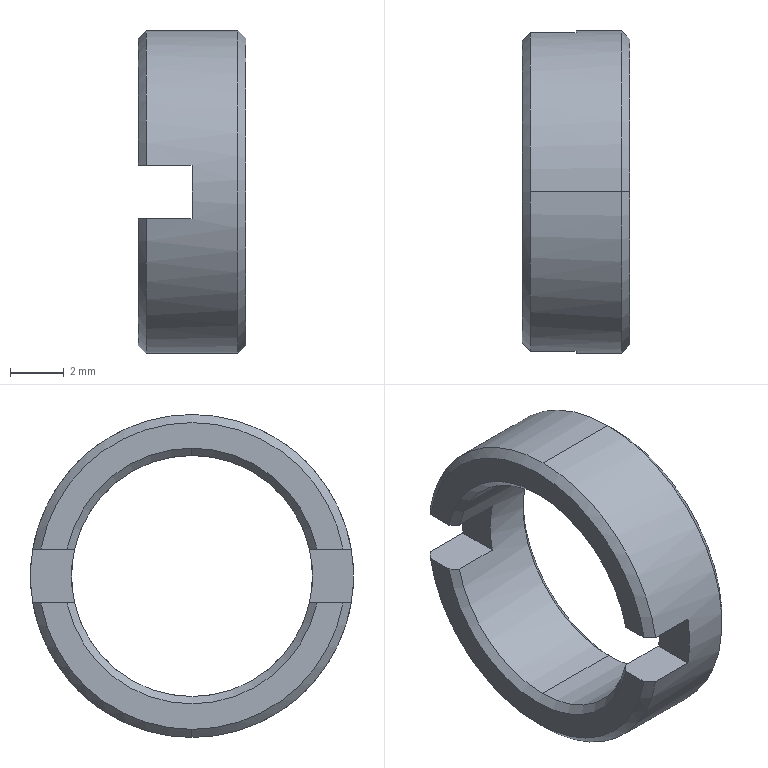Part | SolidWorks | features ICE 1, Revolution 1 | 1 solid | 23 faces | box 4 x 12 x 12 mm | volume 182.884 mm3 | cone 10 | plane 9 | cylinder 4 | commonest cylinder face diameters 8.959 x2 12 x2
STEP:
#1=CARTESIAN_POINT('',(1.7,0.,6.));
#2=VERTEX_POINT('',#1);
#3=CARTESIAN_POINT('',(1.7,0.,-6.));
#4=VERTEX_POINT('',#3);
#5=CARTESIAN_POINT('',(1.7,0.,0.));
#6=DIRECTION('',(-1.,0.,0.));
#7=DIRECTION('',(0.,0.,1.));
#8=AXIS2_PLACEMENT_3D('',#5,#6,#7);
#9=CIRCLE('',#8,6.);
#10=EDGE_CURVE('',#2,#4,#9,.T.);
#11=ORIENTED_EDGE('',*,*,#10,.T.);
#12=CARTESIAN_POINT('',(-1.7,0.,-6.));
#13=VERTEX_POINT('',#12);
#14=CARTESIAN_POINT('',(2.,0.,-6.));
#15=DIRECTION('',(-1.,0.,0.));
#16=VECTOR('',#15,1000.);
#17=LINE('',#14,#16);
#18=EDGE_CURVE('',#4,#13,#17,.T.);
#19=ORIENTED_EDGE('',*,*,#18,.T.);
#20=CARTESIAN_POINT('',(-1.7,5.916,-1.));
#21=VERTEX_POINT('',#20);
#22=CARTESIAN_POINT('',(-1.7,0.,0.));
#23=DIRECTION('',(-1.,0.,0.));
#24=DIRECTION('',(0.,0.,1.));
#25=AXIS2_PLACEMENT_3D('',#22,#23,#24);
#26=CIRCLE('',#25,6.);
#27=EDGE_CURVE('',#21,#13,#26,.T.);
#28=ORIENTED_EDGE('',*,*,#27,.F.);
#29=CARTESIAN_POINT('',(0.,5.916,-1.));
#30=VERTEX_POINT('',#29);
#31=CARTESIAN_POINT('',(2.,5.916,-1.));
#32=DIRECTION('',(-1.,0.,0.));
#33=VECTOR('',#32,1000.);
#34=LINE('',#31,#33);
#35=EDGE_CURVE('',#30,#21,#34,.T.);
#36=ORIENTED_EDGE('',*,*,#35,.F.);
#37=CARTESIAN_POINT('',(0.,5.916,1.));
#38=VERTEX_POINT('',#37);
#39=CARTESIAN_POINT('',(0.,0.,0.));
#40=DIRECTION('',(-1.,0.,0.));
#41=DIRECTION('',(0.,0.,1.));
#42=AXIS2_PLACEMENT_3D('',#39,#40,#41);
#43=CIRCLE('',#42,6.);
#44=EDGE_CURVE('',#38,#30,#43,.T.);
#45=ORIENTED_EDGE('',*,*,#44,.F.);
#46=CARTESIAN_POINT('',(-1.7,5.916,1.));
#47=VERTEX_POINT('',#46);
#48=CARTESIAN_POINT('',(2.,5.916,1.));
#49=DIRECTION('',(-1.,0.,0.));
#50=VECTOR('',#49,1000.);
#51=LINE('',#48,#50);
#52=EDGE_CURVE('',#38,#47,#51,.T.);
#53=ORIENTED_EDGE('',*,*,#52,.T.);
#54=CARTESIAN_POINT('',(-1.7,0.,6.));
#55=VERTEX_POINT('',#54);
#56=CARTESIAN_POINT('',(-1.7,0.,0.));
#57=DIRECTION('',(-1.,0.,0.));
#58=DIRECTION('',(0.,0.,1.));
#59=AXIS2_PLACEMENT_3D('',#56,#57,#58);
#60=CIRCLE('',#59,6.);
#61=EDGE_CURVE('',#55,#47,#60,.T.);
#62=ORIENTED_EDGE('',*,*,#61,.F.);
#63=CARTESIAN_POINT('',(2.,0.,6.));
#64=DIRECTION('',(-1.,0.,0.));
#65=VECTOR('',#64,1000.);
#66=LINE('',#63,#65);
#67=EDGE_CURVE('',#2,#55,#66,.T.);
#68=ORIENTED_EDGE('',*,*,#67,.F.);
#69=EDGE_LOOP('',(#11,#19,#28,#36,#45,#53,#62,#68));
#70=FACE_OUTER_BOUND('',#69,.T.);
#71=CARTESIAN_POINT('',(2.,0.,0.));
#72=DIRECTION('',(-1.,0.,0.));
#73=DIRECTION('',(0.,0.,1.));
#74=AXIS2_PLACEMENT_3D('',#71,#72,#73);
#75=CYLINDRICAL_SURFACE('',#74,6.);
#76=ADVANCED_FACE('',(#70),#75,.T.);
#77=CARTESIAN_POINT('',(2.,0.,5.7));
#78=VERTEX_POINT('',#77);
#79=CARTESIAN_POINT('',(2.,0.,-5.7));
#80=VERTEX_POINT('',#79);
#81=CARTESIAN_POINT('',(2.,0.,0.));
#82=DIRECTION('',(-1.,0.,0.));
#83=DIRECTION('',(0.,0.,1.));
#84=AXIS2_PLACEMENT_3D('',#81,#82,#83);
#85=CIRCLE('',#84,5.7);
#86=EDGE_CURVE('',#78,#80,#85,.T.);
#87=ORIENTED_EDGE('',*,*,#86,.T.);
#88=CARTESIAN_POINT('',(2.,0.,-5.7));
#89=DIRECTION('',(-0.7071,0.,-0.7071));
#90=VECTOR('',#89,1000.);
#91=LINE('',#88,#90);
#92=EDGE_CURVE('',#80,#4,#91,.T.);
#93=ORIENTED_EDGE('',*,*,#92,.T.);
#94=ORIENTED_EDGE('',*,*,#10,.F.);
#95=CARTESIAN_POINT('',(2.,0.,5.7));
#96=DIRECTION('',(-0.7071,0.,0.7071));
#97=VECTOR('',#96,1000.);
#98=LINE('',#95,#97);
#99=EDGE_CURVE('',#78,#2,#98,.T.);
#100=ORIENTED_EDGE('',*,*,#99,.F.);
#101=EDGE_LOOP('',(#87,#93,#94,#100));
#102=FACE_OUTER_BOUND('',#101,.T.);
#103=CARTESIAN_POINT('',(2.,0.,0.));
#104=DIRECTION('',(-1.,0.,0.));
#105=DIRECTION('',(0.,0.,1.));
#106=AXIS2_PLACEMENT_3D('',#103,#104,#105);
#107=CONICAL_SURFACE('',#106,5.7,0.7854);
#108=ADVANCED_FACE('',(#102),#107,.T.);
#109=CARTESIAN_POINT('',(1.729,0.,-4.479));
#110=VERTEX_POINT('',#109);
#111=CARTESIAN_POINT('',(1.729,0.,4.479));
#112=VERTEX_POINT('',#111);
#113=CARTESIAN_POINT('',(1.729,0.,0.));
#114=DIRECTION('',(-1.,0.,0.));
#115=DIRECTION('',(0.,0.,1.));
#116=AXIS2_PLACEMENT_3D('',#113,#114,#115);
#117=CIRCLE('',#116,4.479);
#118=EDGE_CURVE('',#110,#112,#117,.T.);
#119=ORIENTED_EDGE('',*,*,#118,.T.);
#120=CARTESIAN_POINT('',(2.,0.,4.75));
#121=VERTEX_POINT('',#120);
#122=CARTESIAN_POINT('',(1.729,0.,4.479));
#123=DIRECTION('',(0.7071,0.,0.7071));
#124=VECTOR('',#123,1000.);
#125=LINE('',#122,#124);
#126=EDGE_CURVE('',#112,#121,#125,.T.);
#127=ORIENTED_EDGE('',*,*,#126,.T.);
#128=CARTESIAN_POINT('',(2.,0.,-4.75));
#129=VERTEX_POINT('',#128);
#130=CARTESIAN_POINT('',(2.,0.,0.));
#131=DIRECTION('',(-1.,0.,0.));
#132=DIRECTION('',(0.,0.,1.));
#133=AXIS2_PLACEMENT_3D('',#130,#131,#132);
#134=CIRCLE('',#133,4.75);
#135=EDGE_CURVE('',#129,#121,#134,.T.);
#136=ORIENTED_EDGE('',*,*,#135,.F.);
#137=CARTESIAN_POINT('',(1.729,0.,-4.479));
#138=DIRECTION('',(0.7071,0.,-0.7071));
#139=VECTOR('',#138,1000.);
#140=LINE('',#137,#139);
#141=EDGE_CURVE('',#110,#129,#140,.T.);
#142=ORIENTED_EDGE('',*,*,#141,.F.);
#143=EDGE_LOOP('',(#119,#127,#136,#142));
#144=FACE_OUTER_BOUND('',#143,.T.);
#145=CARTESIAN_POINT('',(1.729,0.,0.));
#146=DIRECTION('',(1.,0.,0.));
#147=DIRECTION('',(0.,0.,-1.));
#148=AXIS2_PLACEMENT_3D('',#145,#146,#147);
#149=CONICAL_SURFACE('',#148,4.479,0.7854);
#150=ADVANCED_FACE('',(#144),#149,.F.);
#151=ORIENTED_EDGE('',*,*,#118,.F.);
#152=CARTESIAN_POINT('',(-1.73,0.,-4.479));
#153=VERTEX_POINT('',#152);
#154=CARTESIAN_POINT('',(2.,0.,-4.479));
#155=DIRECTION('',(-1.,0.,0.));
#156=VECTOR('',#155,1000.);
#157=LINE('',#154,#156);
#158=EDGE_CURVE('',#110,#153,#157,.T.);
#159=ORIENTED_EDGE('',*,*,#158,.T.);
#160=CARTESIAN_POINT('',(-1.73,-4.366,-1.));
#161=VERTEX_POINT('',#160);
#162=CARTESIAN_POINT('',(-1.73,0.,0.));
#163=DIRECTION('',(-1.,0.,0.));
#164=DIRECTION('',(0.,0.,1.));
#165=AXIS2_PLACEMENT_3D('',#162,#163,#164);
#166=CIRCLE('',#165,4.479);
#167=EDGE_CURVE('',#153,#161,#166,.T.);
#168=ORIENTED_EDGE('',*,*,#167,.T.);
#169=CARTESIAN_POINT('',(0.,-4.366,-1.));
#170=VERTEX_POINT('',#169);
#171=CARTESIAN_POINT('',(2.,-4.366,-1.));
#172=DIRECTION('',(-1.,0.,0.));
#173=VECTOR('',#172,1000.);
#174=LINE('',#171,#173);
#175=EDGE_CURVE('',#170,#161,#174,.T.);
#176=ORIENTED_EDGE('',*,*,#175,.F.);
#177=CARTESIAN_POINT('',(0.,-4.366,1.));
#178=VERTEX_POINT('',#177);
#179=CARTESIAN_POINT('',(0.,0.,0.));
#180=DIRECTION('',(1.,0.,0.));
#181=DIRECTION('',(0.,0.,1.));
#182=AXIS2_PLACEMENT_3D('',#179,#180,#181);
#183=CIRCLE('',#182,4.479);
#184=EDGE_CURVE('',#178,#170,#183,.T.);
#185=ORIENTED_EDGE('',*,*,#184,.F.);
#186=CARTESIAN_POINT('',(-1.73,-4.366,1.));
#187=VERTEX_POINT('',#186);
#188=CARTESIAN_POINT('',(2.,-4.366,1.));
#189=DIRECTION('',(-1.,0.,0.));
#190=VECTOR('',#189,1000.);
#191=LINE('',#188,#190);
#192=EDGE_CURVE('',#178,#187,#191,.T.);
#193=ORIENTED_EDGE('',*,*,#192,.T.);
#194=CARTESIAN_POINT('',(-1.73,0.,4.479));
#195=VERTEX_POINT('',#194);
#196=CARTESIAN_POINT('',(-1.73,0.,0.));
#197=DIRECTION('',(-1.,0.,0.));
#198=DIRECTION('',(0.,0.,1.));
#199=AXIS2_PLACEMENT_3D('',#196,#197,#198);
#200=CIRCLE('',#199,4.479);
#201=EDGE_CURVE('',#187,#195,#200,.T.);
#202=ORIENTED_EDGE('',*,*,#201,.T.);
#203=CARTESIAN_POINT('',(2.,0.,4.479));
#204=DIRECTION('',(-1.,0.,0.));
#205=VECTOR('',#204,1000.);
#206=LINE('',#203,#205);
#207=EDGE_CURVE('',#112,#195,#206,.T.);
#208=ORIENTED_EDGE('',*,*,#207,.F.);
#209=EDGE_LOOP('',(#151,#159,#168,#176,#185,#193,#202,#208));
#210=FACE_OUTER_BOUND('',#209,.T.);
#211=CARTESIAN_POINT('',(2.,0.,0.));
#212=DIRECTION('',(-1.,0.,0.));
#213=DIRECTION('',(0.,0.,1.));
#214=AXIS2_PLACEMENT_3D('',#211,#212,#213);
#215=CYLINDRICAL_SURFACE('',#214,4.479);
#216=ADVANCED_FACE('',(#210),#215,.F.);
#217=CARTESIAN_POINT('',(-1.73,4.366,1.));
#218=VERTEX_POINT('',#217);
#219=CARTESIAN_POINT('',(-1.73,0.,0.));
#220=DIRECTION('',(-1.,0.,0.));
#221=DIRECTION('',(0.,0.,1.));
#222=AXIS2_PLACEMENT_3D('',#219,#220,#221);
#223=CIRCLE('',#222,4.479);
#224=EDGE_CURVE('',#195,#218,#223,.T.);
#225=ORIENTED_EDGE('',*,*,#224,.F.);
#226=CARTESIAN_POINT('',(-2.,0.,4.75));
#227=VERTEX_POINT('',#226);
#228=CARTESIAN_POINT('',(-2.,0.,4.75));
#229=DIRECTION('',(-0.7071,0.,0.7071));
#230=VECTOR('',#229,1000.);
#231=LINE('',#228,#230);
#232=EDGE_CURVE('',#195,#227,#231,.T.);
#233=ORIENTED_EDGE('',*,*,#232,.T.);
#234=CARTESIAN_POINT('',(-2.,4.644,1.));
#235=VERTEX_POINT('',#234);
#236=CARTESIAN_POINT('',(-2.,0.,0.));
#237=DIRECTION('',(-1.,0.,0.));
#238=DIRECTION('',(0.,0.,1.));
#239=AXIS2_PLACEMENT_3D('',#236,#237,#238);
#240=CIRCLE('',#239,4.75);
#241=EDGE_CURVE('',#227,#235,#240,.T.);
#242=ORIENTED_EDGE('',*,*,#241,.T.);
#243=CARTESIAN_POINT('',(-2.,4.644,1.));
#244=CARTESIAN_POINT('',(-1.91,4.551,1.));
#245=CARTESIAN_POINT('',(-1.82,4.459,1.));
#246=CARTESIAN_POINT('',(-1.73,4.366,1.));
#247=B_SPLINE_CURVE_WITH_KNOTS('',3,(#243,#244,#245,#246),.UNSPECIFIED.,.F.,.F.,(4,4),(0.000001,0.0003876),.UNSPECIFIED.);
#248=EDGE_CURVE('',#235,#218,#247,.T.);
#249=ORIENTED_EDGE('',*,*,#248,.T.);
#250=EDGE_LOOP('',(#225,#233,#242,#249));
#251=FACE_OUTER_BOUND('',#250,.T.);
#252=CARTESIAN_POINT('',(-2.,0.,0.));
#253=DIRECTION('',(-1.,0.,0.));
#254=DIRECTION('',(0.,0.,1.));
#255=AXIS2_PLACEMENT_3D('',#252,#253,#254);
#256=CONICAL_SURFACE('',#255,4.75,0.7854);
#257=ADVANCED_FACE('',(#251),#256,.F.);
#258=CARTESIAN_POINT('',(-2.,0.,-5.7));
#259=VERTEX_POINT('',#258);
#260=CARTESIAN_POINT('',(-2.,-5.612,-1.));
#261=VERTEX_POINT('',#260);
#262=CARTESIAN_POINT('',(-2.,0.,0.));
#263=DIRECTION('',(-1.,0.,0.));
#264=DIRECTION('',(0.,0.,1.));
#265=AXIS2_PLACEMENT_3D('',#262,#263,#264);
#266=CIRCLE('',#265,5.7);
#267=EDGE_CURVE('',#259,#261,#266,.T.);
#268=ORIENTED_EDGE('',*,*,#267,.F.);
#269=CARTESIAN_POINT('',(-1.7,0.,-6.));
#270=DIRECTION('',(0.7071,0.,-0.7071));
#271=VECTOR('',#270,1000.);
#272=LINE('',#269,#271);
#273=EDGE_CURVE('',#259,#13,#272,.T.);
#274=ORIENTED_EDGE('',*,*,#273,.T.);
#275=CARTESIAN_POINT('',(-1.7,-5.916,-1.));
#276=VERTEX_POINT('',#275);
#277=CARTESIAN_POINT('',(-1.7,0.,0.));
#278=DIRECTION('',(-1.,0.,0.));
#279=DIRECTION('',(0.,0.,1.));
#280=AXIS2_PLACEMENT_3D('',#277,#278,#279);
#281=CIRCLE('',#280,6.);
#282=EDGE_CURVE('',#13,#276,#281,.T.);
#283=ORIENTED_EDGE('',*,*,#282,.T.);
#284=CARTESIAN_POINT('',(-2.,-5.612,-1.));
#285=CARTESIAN_POINT('',(-1.9,-5.713,-1.));
#286=CARTESIAN_POINT('',(-1.8,-5.815,-1.));
#287=CARTESIAN_POINT('',(-1.7,-5.916,-1.));
#288=B_SPLINE_CURVE_WITH_KNOTS('',3,(#284,#285,#286,#287),.UNSPECIFIED.,.F.,.F.,(4,4),(0.01512,0.01555),.UNSPECIFIED.);
#289=EDGE_CURVE('',#261,#276,#288,.T.);
#290=ORIENTED_EDGE('',*,*,#289,.F.);
#291=EDGE_LOOP('',(#268,#274,#283,#290));
#292=FACE_OUTER_BOUND('',#291,.T.);
#293=CARTESIAN_POINT('',(-1.7,0.,0.));
#294=DIRECTION('',(1.,0.,0.));
#295=DIRECTION('',(0.,0.,-1.));
#296=AXIS2_PLACEMENT_3D('',#293,#294,#295);
#297=CONICAL_SURFACE('',#296,6.,0.7854);
#298=ADVANCED_FACE('',(#292),#297,.T.);
#299=CARTESIAN_POINT('',(-2.,5.612,-1.));
#300=VERTEX_POINT('',#299);
#301=CARTESIAN_POINT('',(-2.,4.644,-1.));
#302=VERTEX_POINT('',#301);
#303=CARTESIAN_POINT('',(-2.,5.7,-1.));
#304=DIRECTION('',(0.,-1.,0.));
#305=VECTOR('',#304,1000.);
#306=LINE('',#303,#305);
#307=EDGE_CURVE('',#300,#302,#306,.T.);
#308=ORIENTED_EDGE('',*,*,#307,.F.);
#309=CARTESIAN_POINT('',(-2.,0.,0.));
#310=DIRECTION('',(-1.,0.,0.));
#311=DIRECTION('',(0.,0.,1.));
#312=AXIS2_PLACEMENT_3D('',#309,#310,#311);
#313=CIRCLE('',#312,5.7);
#314=EDGE_CURVE('',#300,#259,#313,.T.);
#315=ORIENTED_EDGE('',*,*,#314,.T.);
#316=ORIENTED_EDGE('',*,*,#267,.T.);
#317=CARTESIAN_POINT('',(-2.,-4.644,-1.));
#318=VERTEX_POINT('',#317);
#319=CARTESIAN_POINT('',(-2.,5.7,-1.));
#320=DIRECTION('',(0.,-1.,0.));
#321=VECTOR('',#320,1000.);
#322=LINE('',#319,#321);
#323=EDGE_CURVE('',#318,#261,#322,.T.);
#324=ORIENTED_EDGE('',*,*,#323,.F.);
#325=CARTESIAN_POINT('',(-2.,0.,0.));
#326=DIRECTION('',(-1.,0.,0.));
#327=DIRECTION('',(0.,0.,1.));
#328=AXIS2_PLACEMENT_3D('',#325,#326,#327);
#329=CIRCLE('',#328,4.75);
#330=EDGE_CURVE('',#302,#318,#329,.T.);
#331=ORIENTED_EDGE('',*,*,#330,.F.);
#332=EDGE_LOOP('',(#308,#315,#316,#324,#331));
#333=FACE_OUTER_BOUND('',#332,.T.);
#334=CARTESIAN_POINT('',(-2.,5.7,0.));
#335=DIRECTION('',(1.,0.,0.));
#336=DIRECTION('',(0.,0.,-1.));
#337=AXIS2_PLACEMENT_3D('',#334,#335,#336);
#338=PLANE('',#337);
#339=ADVANCED_FACE('',(#333),#338,.F.);
#340=CARTESIAN_POINT('',(-1.73,4.366,-1.));
#341=VERTEX_POINT('',#340);
#342=CARTESIAN_POINT('',(-2.,4.644,-1.));
#343=CARTESIAN_POINT('',(-1.91,4.551,-1.));
#344=CARTESIAN_POINT('',(-1.82,4.459,-1.));
#345=CARTESIAN_POINT('',(-1.73,4.366,-1.));
#346=B_SPLINE_CURVE_WITH_KNOTS('',3,(#342,#343,#344,#345),.UNSPECIFIED.,.F.,.F.,(4,4),(0.000001,0.0003876),.UNSPECIFIED.);
#347=EDGE_CURVE('',#302,#341,#346,.T.);
#348=ORIENTED_EDGE('',*,*,#347,.F.);
#349=ORIENTED_EDGE('',*,*,#330,.T.);
#350=CARTESIAN_POINT('',(-1.73,-4.366,-1.));
#351=CARTESIAN_POINT('',(-1.82,-4.459,-1.));
#352=CARTESIAN_POINT('',(-1.91,-4.551,-1.));
#353=CARTESIAN_POINT('',(-2.,-4.644,-1.));
#354=B_SPLINE_CURVE_WITH_KNOTS('',3,(#350,#351,#352,#353),.UNSPECIFIED.,.F.,.F.,(4,4),(0.01142,0.01179),.UNSPECIFIED.);
#355=EDGE_CURVE('',#161,#318,#354,.T.);
#356=ORIENTED_EDGE('',*,*,#355,.F.);
#357=ORIENTED_EDGE('',*,*,#167,.F.);
#358=CARTESIAN_POINT('',(-1.73,0.,0.));
#359=DIRECTION('',(-1.,0.,0.));
#360=DIRECTION('',(0.,0.,1.));
#361=AXIS2_PLACEMENT_3D('',#358,#359,#360);
#362=CIRCLE('',#361,4.479);
#363=EDGE_CURVE('',#341,#153,#362,.T.);
#364=ORIENTED_EDGE('',*,*,#363,.F.);
#365=EDGE_LOOP('',(#348,#349,#356,#357,#364));
#366=FACE_OUTER_BOUND('',#365,.T.);
#367=CARTESIAN_POINT('',(-2.,0.,0.));
#368=DIRECTION('',(-1.,0.,0.));
#369=DIRECTION('',(0.,0.,1.));
#370=AXIS2_PLACEMENT_3D('',#367,#368,#369);
#371=CONICAL_SURFACE('',#370,4.75,0.7854);
#372=ADVANCED_FACE('',(#366),#371,.F.);
#373=ORIENTED_EDGE('',*,*,#273,.F.);
#374=ORIENTED_EDGE('',*,*,#314,.F.);
#375=CARTESIAN_POINT('',(-1.7,5.916,-1.));
#376=CARTESIAN_POINT('',(-1.8,5.815,-1.));
#377=CARTESIAN_POINT('',(-1.9,5.713,-1.));
#378=CARTESIAN_POINT('',(-2.,5.612,-1.));
#379=B_SPLINE_CURVE_WITH_KNOTS('',3,(#375,#376,#377,#378),.UNSPECIFIED.,.F.,.F.,(4,4),(0.000000996,0.0004282),.UNSPECIFIED.);
#380=EDGE_CURVE('',#21,#300,#379,.T.);
#381=ORIENTED_EDGE('',*,*,#380,.F.);
#382=ORIENTED_EDGE('',*,*,#27,.T.);
#383=EDGE_LOOP('',(#373,#374,#381,#382));
#384=FACE_OUTER_BOUND('',#383,.T.);
#385=CARTESIAN_POINT('',(-1.7,0.,0.));
#386=DIRECTION('',(1.,0.,0.));
#387=DIRECTION('',(0.,0.,-1.));
#388=AXIS2_PLACEMENT_3D('',#385,#386,#387);
#389=CONICAL_SURFACE('',#388,6.,0.7854);
#390=ADVANCED_FACE('',(#384),#389,.T.);
#391=CARTESIAN_POINT('',(-2.,-5.612,1.));
#392=VERTEX_POINT('',#391);
#393=CARTESIAN_POINT('',(-2.,5.612,1.));
#394=VERTEX_POINT('',#393);
#395=CARTESIAN_POINT('',(-2.,0.,0.));
#396=DIRECTION('',(-1.,0.,0.));
#397=DIRECTION('',(0.,0.,1.));
#398=AXIS2_PLACEMENT_3D('',#395,#396,#397);
#399=CIRCLE('',#398,5.7);
#400=EDGE_CURVE('',#392,#394,#399,.T.);
#401=ORIENTED_EDGE('',*,*,#400,.T.);
#402=CARTESIAN_POINT('',(-2.,5.7,1.));
#403=DIRECTION('',(0.,-1.,0.));
#404=VECTOR('',#403,1000.);
#405=LINE('',#402,#404);
#406=EDGE_CURVE('',#394,#235,#405,.T.);
#407=ORIENTED_EDGE('',*,*,#406,.T.);
#408=ORIENTED_EDGE('',*,*,#241,.F.);
#409=CARTESIAN_POINT('',(-2.,-4.644,1.));
#410=VERTEX_POINT('',#409);
#411=CARTESIAN_POINT('',(-2.,0.,0.));
#412=DIRECTION('',(-1.,0.,0.));
#413=DIRECTION('',(0.,0.,1.));
#414=AXIS2_PLACEMENT_3D('',#411,#412,#413);
#415=CIRCLE('',#414,4.75);
#416=EDGE_CURVE('',#410,#227,#415,.T.);
#417=ORIENTED_EDGE('',*,*,#416,.F.);
#418=CARTESIAN_POINT('',(-2.,5.7,1.));
#419=DIRECTION('',(0.,-1.,0.));
#420=VECTOR('',#419,1000.);
#421=LINE('',#418,#420);
#422=EDGE_CURVE('',#410,#392,#421,.T.);
#423=ORIENTED_EDGE('',*,*,#422,.T.);
#424=EDGE_LOOP('',(#401,#407,#408,#417,#423));
#425=FACE_OUTER_BOUND('',#424,.T.);
#426=CARTESIAN_POINT('',(-2.,5.7,0.));
#427=DIRECTION('',(1.,0.,0.));
#428=DIRECTION('',(0.,0.,-1.));
#429=AXIS2_PLACEMENT_3D('',#426,#427,#428);
#430=PLANE('',#429);
#431=ADVANCED_FACE('',(#425),#430,.F.);
#432=ORIENTED_EDGE('',*,*,#232,.F.);
#433=ORIENTED_EDGE('',*,*,#201,.F.);
#434=CARTESIAN_POINT('',(-1.73,-4.366,1.));
#435=CARTESIAN_POINT('',(-1.82,-4.459,1.));
#436=CARTESIAN_POINT('',(-1.91,-4.551,1.));
#437=CARTESIAN_POINT('',(-2.,-4.644,1.));
#438=B_SPLINE_CURVE_WITH_KNOTS('',3,(#434,#435,#436,#437),.UNSPECIFIED.,.F.,.F.,(4,4),(0.01142,0.01179),.UNSPECIFIED.);
#439=EDGE_CURVE('',#187,#410,#438,.T.);
#440=ORIENTED_EDGE('',*,*,#439,.T.);
#441=ORIENTED_EDGE('',*,*,#416,.T.);
#442=EDGE_LOOP('',(#432,#433,#440,#441));
#443=FACE_OUTER_BOUND('',#442,.T.);
#444=CARTESIAN_POINT('',(-2.,0.,0.));
#445=DIRECTION('',(-1.,0.,0.));
#446=DIRECTION('',(0.,0.,1.));
#447=AXIS2_PLACEMENT_3D('',#444,#445,#446);
#448=CONICAL_SURFACE('',#447,4.75,0.7854);
#449=ADVANCED_FACE('',(#443),#448,.F.);
#450=ORIENTED_EDGE('',*,*,#158,.F.);
#451=CARTESIAN_POINT('',(1.729,0.,0.));
#452=DIRECTION('',(-1.,0.,0.));
#453=DIRECTION('',(0.,0.,1.));
#454=AXIS2_PLACEMENT_3D('',#451,#452,#453);
#455=CIRCLE('',#454,4.479);
#456=EDGE_CURVE('',#112,#110,#455,.T.);
#457=ORIENTED_EDGE('',*,*,#456,.F.);
#458=ORIENTED_EDGE('',*,*,#207,.T.);
#459=ORIENTED_EDGE('',*,*,#224,.T.);
#460=CARTESIAN_POINT('',(0.,4.366,1.));
#461=VERTEX_POINT('',#460);
#462=CARTESIAN_POINT('',(2.,4.366,1.));
#463=DIRECTION('',(1.,0.,0.));
#464=VECTOR('',#463,1000.);
#465=LINE('',#462,#464);
#466=EDGE_CURVE('',#218,#461,#465,.T.);
#467=ORIENTED_EDGE('',*,*,#466,.T.);
#468=CARTESIAN_POINT('',(0.,4.366,-1.));
#469=VERTEX_POINT('',#468);
#470=CARTESIAN_POINT('',(0.,0.,0.));
#471=DIRECTION('',(1.,0.,0.));
#472=DIRECTION('',(0.,0.,1.));
#473=AXIS2_PLACEMENT_3D('',#470,#471,#472);
#474=CIRCLE('',#473,4.479);
#475=EDGE_CURVE('',#469,#461,#474,.T.);
#476=ORIENTED_EDGE('',*,*,#475,.F.);
#477=CARTESIAN_POINT('',(2.,4.366,-1.));
#478=DIRECTION('',(1.,0.,0.));
#479=VECTOR('',#478,1000.);
#480=LINE('',#477,#479);
#481=EDGE_CURVE('',#341,#469,#480,.T.);
#482=ORIENTED_EDGE('',*,*,#481,.F.);
#483=ORIENTED_EDGE('',*,*,#363,.T.);
#484=EDGE_LOOP('',(#450,#457,#458,#459,#467,#476,#482,#483));
#485=FACE_OUTER_BOUND('',#484,.T.);
#486=CARTESIAN_POINT('',(2.,0.,0.));
#487=DIRECTION('',(-1.,0.,0.));
#488=DIRECTION('',(0.,0.,1.));
#489=AXIS2_PLACEMENT_3D('',#486,#487,#488);
#490=CYLINDRICAL_SURFACE('',#489,4.479);
#491=ADVANCED_FACE('',(#485),#490,.F.);
#492=ORIENTED_EDGE('',*,*,#126,.F.);
#493=ORIENTED_EDGE('',*,*,#456,.T.);
#494=ORIENTED_EDGE('',*,*,#141,.T.);
#495=CARTESIAN_POINT('',(2.,0.,0.));
#496=DIRECTION('',(-1.,0.,0.));
#497=DIRECTION('',(0.,0.,1.));
#498=AXIS2_PLACEMENT_3D('',#495,#496,#497);
#499=CIRCLE('',#498,4.75);
#500=EDGE_CURVE('',#121,#129,#499,.T.);
#501=ORIENTED_EDGE('',*,*,#500,.F.);
#502=EDGE_LOOP('',(#492,#493,#494,#501));
#503=FACE_OUTER_BOUND('',#502,.T.);
#504=CARTESIAN_POINT('',(1.729,0.,0.));
#505=DIRECTION('',(1.,0.,0.));
#506=DIRECTION('',(0.,0.,-1.));
#507=AXIS2_PLACEMENT_3D('',#504,#505,#506);
#508=CONICAL_SURFACE('',#507,4.479,0.7854);
#509=ADVANCED_FACE('',(#503),#508,.F.);
#510=ORIENTED_EDGE('',*,*,#86,.F.);
#511=CARTESIAN_POINT('',(2.,0.,0.));
#512=DIRECTION('',(-1.,0.,0.));
#513=DIRECTION('',(0.,0.,1.));
#514=AXIS2_PLACEMENT_3D('',#511,#512,#513);
#515=CIRCLE('',#514,5.7);
#516=EDGE_CURVE('',#80,#78,#515,.T.);
#517=ORIENTED_EDGE('',*,*,#516,.F.);
#518=EDGE_LOOP('',(#510,#517));
#519=FACE_OUTER_BOUND('',#518,.T.);
#520=ORIENTED_EDGE('',*,*,#135,.T.);
#521=ORIENTED_EDGE('',*,*,#500,.T.);
#522=EDGE_LOOP('',(#520,#521));
#523=FACE_BOUND('',#522,.T.);
#524=CARTESIAN_POINT('',(2.,4.75,0.));
#525=DIRECTION('',(-1.,0.,0.));
#526=DIRECTION('',(0.,0.,1.));
#527=AXIS2_PLACEMENT_3D('',#524,#525,#526);
#528=PLANE('',#527);
#529=ADVANCED_FACE('',(#519,#523),#528,.F.);
#530=ORIENTED_EDGE('',*,*,#92,.F.);
#531=ORIENTED_EDGE('',*,*,#516,.T.);
#532=ORIENTED_EDGE('',*,*,#99,.T.);
#533=CARTESIAN_POINT('',(1.7,0.,0.));
#534=DIRECTION('',(-1.,0.,0.));
#535=DIRECTION('',(0.,0.,1.));
#536=AXIS2_PLACEMENT_3D('',#533,#534,#535);
#537=CIRCLE('',#536,6.);
#538=EDGE_CURVE('',#4,#2,#537,.T.);
#539=ORIENTED_EDGE('',*,*,#538,.F.);
#540=EDGE_LOOP('',(#530,#531,#532,#539));
#541=FACE_OUTER_BOUND('',#540,.T.);
#542=CARTESIAN_POINT('',(2.,0.,0.));
#543=DIRECTION('',(-1.,0.,0.));
#544=DIRECTION('',(0.,0.,1.));
#545=AXIS2_PLACEMENT_3D('',#542,#543,#544);
#546=CONICAL_SURFACE('',#545,5.7,0.7854);
#547=ADVANCED_FACE('',(#541),#546,.T.);
#548=ORIENTED_EDGE('',*,*,#18,.F.);
#549=ORIENTED_EDGE('',*,*,#538,.T.);
#550=ORIENTED_EDGE('',*,*,#67,.T.);
#551=CARTESIAN_POINT('',(-1.7,-5.916,1.));
#552=VERTEX_POINT('',#551);
#553=CARTESIAN_POINT('',(-1.7,0.,0.));
#554=DIRECTION('',(-1.,0.,0.));
#555=DIRECTION('',(0.,0.,1.));
#556=AXIS2_PLACEMENT_3D('',#553,#554,#555);
#557=CIRCLE('',#556,6.);
#558=EDGE_CURVE('',#552,#55,#557,.T.);
#559=ORIENTED_EDGE('',*,*,#558,.F.);
#560=CARTESIAN_POINT('',(0.,-5.916,1.));
#561=VERTEX_POINT('',#560);
#562=CARTESIAN_POINT('',(2.,-5.916,1.));
#563=DIRECTION('',(1.,0.,0.));
#564=VECTOR('',#563,1000.);
#565=LINE('',#562,#564);
#566=EDGE_CURVE('',#552,#561,#565,.T.);
#567=ORIENTED_EDGE('',*,*,#566,.T.);
#568=CARTESIAN_POINT('',(0.,-5.916,-1.));
#569=VERTEX_POINT('',#568);
#570=CARTESIAN_POINT('',(0.,0.,0.));
#571=DIRECTION('',(-1.,0.,0.));
#572=DIRECTION('',(0.,0.,1.));
#573=AXIS2_PLACEMENT_3D('',#570,#571,#572);
#574=CIRCLE('',#573,6.);
#575=EDGE_CURVE('',#569,#561,#574,.T.);
#576=ORIENTED_EDGE('',*,*,#575,.F.);
#577=CARTESIAN_POINT('',(2.,-5.916,-1.));
#578=DIRECTION('',(1.,0.,0.));
#579=VECTOR('',#578,1000.);
#580=LINE('',#577,#579);
#581=EDGE_CURVE('',#276,#569,#580,.T.);
#582=ORIENTED_EDGE('',*,*,#581,.F.);
#583=ORIENTED_EDGE('',*,*,#282,.F.);
#584=EDGE_LOOP('',(#548,#549,#550,#559,#567,#576,#582,#583));
#585=FACE_OUTER_BOUND('',#584,.T.);
#586=CARTESIAN_POINT('',(2.,0.,0.));
#587=DIRECTION('',(-1.,0.,0.));
#588=DIRECTION('',(0.,0.,1.));
#589=AXIS2_PLACEMENT_3D('',#586,#587,#588);
#590=CYLINDRICAL_SURFACE('',#589,6.);
#591=ADVANCED_FACE('',(#585),#590,.T.);
#592=ORIENTED_EDGE('',*,*,#558,.T.);
#593=ORIENTED_EDGE('',*,*,#61,.T.);
#594=CARTESIAN_POINT('',(-1.7,5.916,1.));
#595=CARTESIAN_POINT('',(-1.8,5.815,1.));
#596=CARTESIAN_POINT('',(-1.9,5.713,1.));
#597=CARTESIAN_POINT('',(-2.,5.612,1.));
#598=B_SPLINE_CURVE_WITH_KNOTS('',3,(#594,#595,#596,#597),.UNSPECIFIED.,.F.,.F.,(4,4),(0.000000996,0.0004282),.UNSPECIFIED.);
#599=EDGE_CURVE('',#47,#394,#598,.T.);
#600=ORIENTED_EDGE('',*,*,#599,.T.);
#601=ORIENTED_EDGE('',*,*,#400,.F.);
#602=CARTESIAN_POINT('',(-2.,-5.612,1.));
#603=CARTESIAN_POINT('',(-1.9,-5.713,1.));
#604=CARTESIAN_POINT('',(-1.8,-5.815,1.));
#605=CARTESIAN_POINT('',(-1.7,-5.916,1.));
#606=B_SPLINE_CURVE_WITH_KNOTS('',3,(#602,#603,#604,#605),.UNSPECIFIED.,.F.,.F.,(4,4),(0.01512,0.01555),.UNSPECIFIED.);
#607=EDGE_CURVE('',#392,#552,#606,.T.);
#608=ORIENTED_EDGE('',*,*,#607,.T.);
#609=EDGE_LOOP('',(#592,#593,#600,#601,#608));
#610=FACE_OUTER_BOUND('',#609,.T.);
#611=CARTESIAN_POINT('',(-1.7,0.,0.));
#612=DIRECTION('',(1.,0.,0.));
#613=DIRECTION('',(0.,0.,-1.));
#614=AXIS2_PLACEMENT_3D('',#611,#612,#613);
#615=CONICAL_SURFACE('',#614,6.,0.7854);
#616=ADVANCED_FACE('',(#610),#615,.T.);
#617=ORIENTED_EDGE('',*,*,#175,.T.);
#618=ORIENTED_EDGE('',*,*,#355,.T.);
#619=ORIENTED_EDGE('',*,*,#323,.T.);
#620=ORIENTED_EDGE('',*,*,#289,.T.);
#621=ORIENTED_EDGE('',*,*,#581,.T.);
#622=CARTESIAN_POINT('',(0.,-10.,-1.));
#623=DIRECTION('',(0.,1.,0.));
#624=VECTOR('',#623,1000.);
#625=LINE('',#622,#624);
#626=EDGE_CURVE('',#569,#170,#625,.T.);
#627=ORIENTED_EDGE('',*,*,#626,.T.);
#628=EDGE_LOOP('',(#617,#618,#619,#620,#621,#627));
#629=FACE_OUTER_BOUND('',#628,.T.);
#630=CARTESIAN_POINT('',(0.,0.,-1.));
#631=DIRECTION('',(0.,0.,1.));
#632=DIRECTION('',(1.,0.,0.));
#633=AXIS2_PLACEMENT_3D('',#630,#631,#632);
#634=PLANE('',#633);
#635=ADVANCED_FACE('',(#629),#634,.T.);
#636=CARTESIAN_POINT('',(0.,-10.,1.));
#637=DIRECTION('',(0.,1.,0.));
#638=VECTOR('',#637,1000.);
#639=LINE('',#636,#638);
#640=EDGE_CURVE('',#561,#178,#639,.T.);
#641=ORIENTED_EDGE('',*,*,#640,.F.);
#642=ORIENTED_EDGE('',*,*,#566,.F.);
#643=ORIENTED_EDGE('',*,*,#607,.F.);
#644=ORIENTED_EDGE('',*,*,#422,.F.);
#645=ORIENTED_EDGE('',*,*,#439,.F.);
#646=ORIENTED_EDGE('',*,*,#192,.F.);
#647=EDGE_LOOP('',(#641,#642,#643,#644,#645,#646));
#648=FACE_OUTER_BOUND('',#647,.T.);
#649=CARTESIAN_POINT('',(0.,0.,1.));
#650=DIRECTION('',(0.,0.,1.));
#651=DIRECTION('',(1.,0.,0.));
#652=AXIS2_PLACEMENT_3D('',#649,#650,#651);
#653=PLANE('',#652);
#654=ADVANCED_FACE('',(#648),#653,.F.);
#655=ORIENTED_EDGE('',*,*,#184,.T.);
#656=ORIENTED_EDGE('',*,*,#626,.F.);
#657=ORIENTED_EDGE('',*,*,#575,.T.);
#658=ORIENTED_EDGE('',*,*,#640,.T.);
#659=EDGE_LOOP('',(#655,#656,#657,#658));
#660=FACE_OUTER_BOUND('',#659,.T.);
#661=CARTESIAN_POINT('',(0.,-10.,1.));
#662=DIRECTION('',(-1.,0.,0.));
#663=DIRECTION('',(0.,0.,1.));
#664=AXIS2_PLACEMENT_3D('',#661,#662,#663);
#665=PLANE('',#664);
#666=ADVANCED_FACE('',(#660),#665,.T.);
#667=ORIENTED_EDGE('',*,*,#475,.T.);
#668=CARTESIAN_POINT('',(0.,-10.,1.));
#669=DIRECTION('',(0.,1.,0.));
#670=VECTOR('',#669,1000.);
#671=LINE('',#668,#670);
#672=EDGE_CURVE('',#461,#38,#671,.T.);
#673=ORIENTED_EDGE('',*,*,#672,.T.);
#674=ORIENTED_EDGE('',*,*,#44,.T.);
#675=CARTESIAN_POINT('',(0.,-10.,-1.));
#676=DIRECTION('',(0.,1.,0.));
#677=VECTOR('',#676,1000.);
#678=LINE('',#675,#677);
#679=EDGE_CURVE('',#469,#30,#678,.T.);
#680=ORIENTED_EDGE('',*,*,#679,.F.);
#681=EDGE_LOOP('',(#667,#673,#674,#680));
#682=FACE_OUTER_BOUND('',#681,.T.);
#683=CARTESIAN_POINT('',(0.,-10.,1.));
#684=DIRECTION('',(-1.,0.,0.));
#685=DIRECTION('',(0.,0.,1.));
#686=AXIS2_PLACEMENT_3D('',#683,#684,#685);
#687=PLANE('',#686);
#688=ADVANCED_FACE('',(#682),#687,.T.);
#689=ORIENTED_EDGE('',*,*,#248,.F.);
#690=ORIENTED_EDGE('',*,*,#406,.F.);
#691=ORIENTED_EDGE('',*,*,#599,.F.);
#692=ORIENTED_EDGE('',*,*,#52,.F.);
#693=ORIENTED_EDGE('',*,*,#672,.F.);
#694=ORIENTED_EDGE('',*,*,#466,.F.);
#695=EDGE_LOOP('',(#689,#690,#691,#692,#693,#694));
#696=FACE_OUTER_BOUND('',#695,.T.);
#697=CARTESIAN_POINT('',(0.,0.,1.));
#698=DIRECTION('',(0.,0.,1.));
#699=DIRECTION('',(1.,0.,0.));
#700=AXIS2_PLACEMENT_3D('',#697,#698,#699);
#701=PLANE('',#700);
#702=ADVANCED_FACE('',(#696),#701,.F.);
#703=ORIENTED_EDGE('',*,*,#481,.T.);
#704=ORIENTED_EDGE('',*,*,#679,.T.);
#705=ORIENTED_EDGE('',*,*,#35,.T.);
#706=ORIENTED_EDGE('',*,*,#380,.T.);
#707=ORIENTED_EDGE('',*,*,#307,.T.);
#708=ORIENTED_EDGE('',*,*,#347,.T.);
#709=EDGE_LOOP('',(#703,#704,#705,#706,#707,#708));
#710=FACE_OUTER_BOUND('',#709,.T.);
#711=CARTESIAN_POINT('',(0.,0.,-1.));
#712=DIRECTION('',(0.,0.,1.));
#713=DIRECTION('',(1.,0.,0.));
#714=AXIS2_PLACEMENT_3D('',#711,#712,#713);
#715=PLANE('',#714);
#716=ADVANCED_FACE('',(#710),#715,.T.);
#717=CLOSED_SHELL('',(#76,#108,#150,#216,#257,#298,#339,#372,#390,#431,#449,#491,#509,#529,#547,#591,#616,#635,#654,#666,#688,#702,#716));
#718=MANIFOLD_SOLID_BREP('',#717);
#719=CARTESIAN_POINT('',(0.,0.,0.));
#720=DIRECTION('',(0.,0.,1.));
#721=DIRECTION('',(1.,0.,0.));
#722=AXIS2_PLACEMENT_3D('',#719,#720,#721);
#723=(LENGTH_UNIT()NAMED_UNIT(*)SI_UNIT(.MILLI.,.METRE.));
#724=UNCERTAINTY_MEASURE_WITH_UNIT(LENGTH_MEASURE(0.00001),#723,'','');
#725=(NAMED_UNIT(*)PLANE_ANGLE_UNIT()SI_UNIT($,.RADIAN.));
#726=(NAMED_UNIT(*)SI_UNIT($,.STERADIAN.)SOLID_ANGLE_UNIT());
#727=(GEOMETRIC_REPRESENTATION_CONTEXT(3)GLOBAL_UNCERTAINTY_ASSIGNED_CONTEXT((#724))GLOBAL_UNIT_ASSIGNED_CONTEXT((#723,#725,#726))REPRESENTATION_CONTEXT('',''));
#728=ADVANCED_BREP_SHAPE_REPRESENTATION('',(#718,#722),#727);